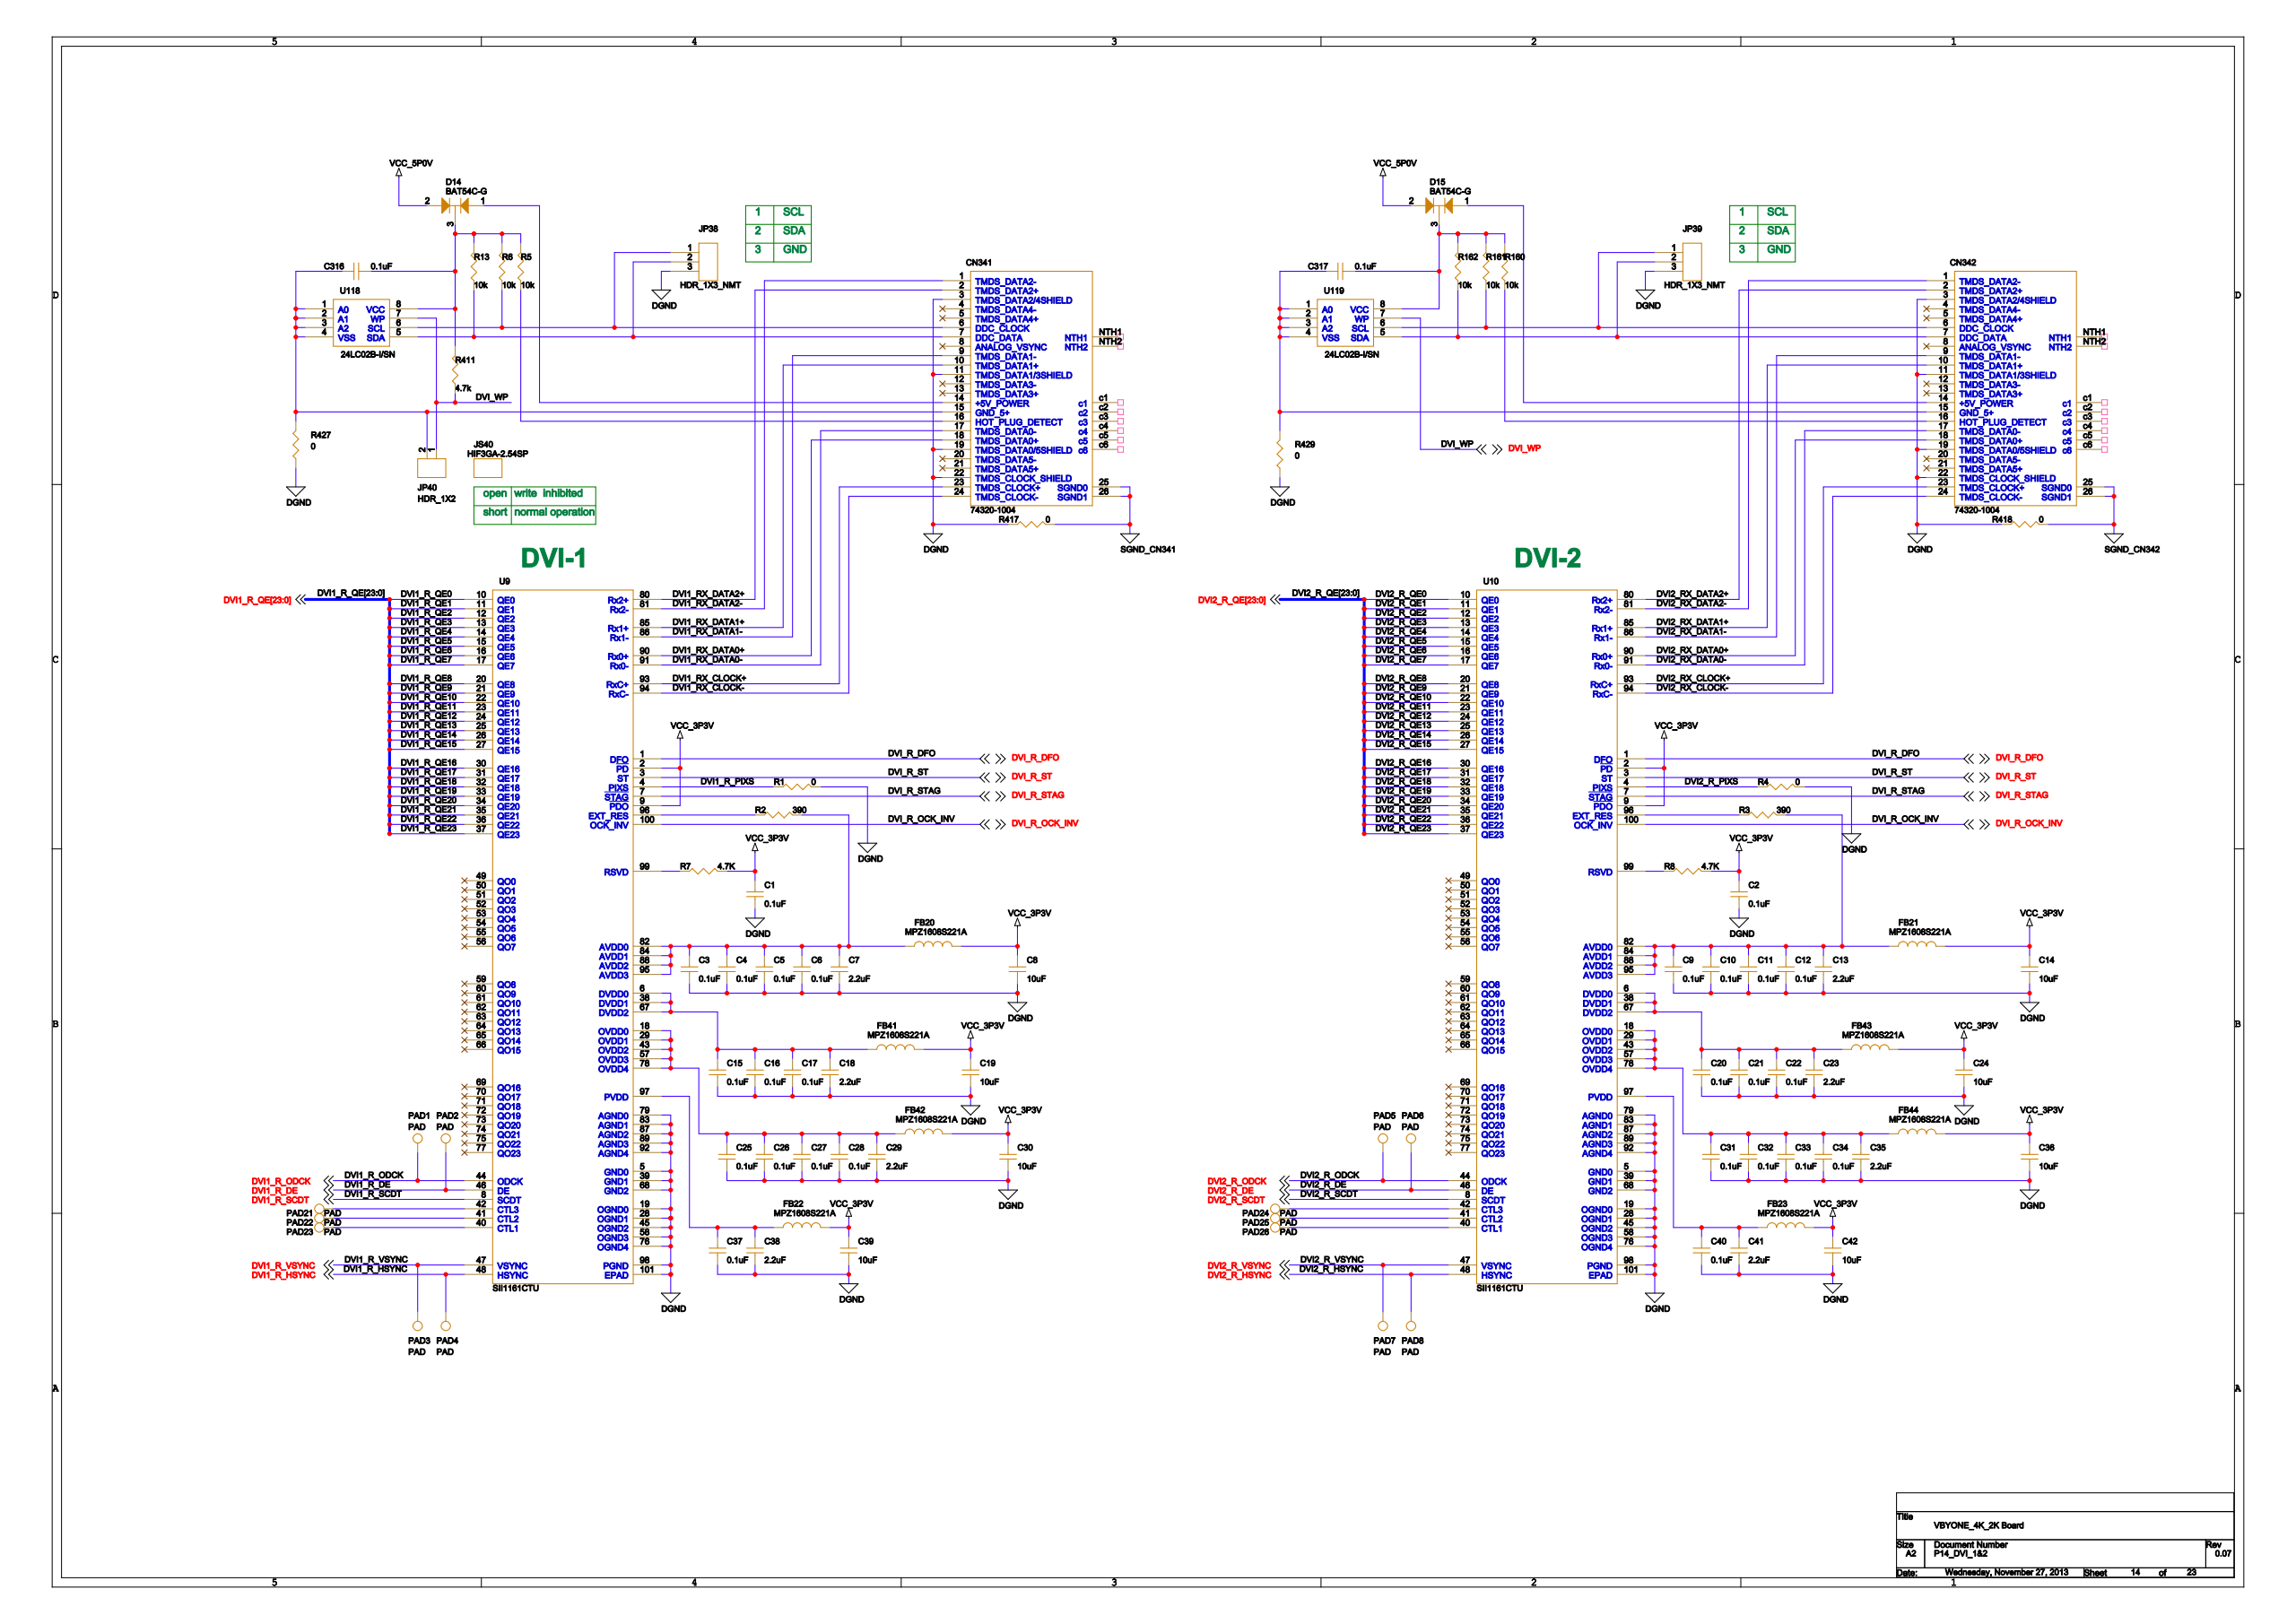Circuit board | Cadence Allegro | 1712 parts | 1495 nets | one sheet of the schematic
Parts on this sheet (reference | value | footprint):
C1 | 0.1uF | CRC1005RZAS
C2 | 0.1uF | CRC1005RZAS
C4 | 0.1uF | CRC1005RZAS
C5 | 0.1uF | CRC1005RZAS
C6 | 0.1uF | CRC1005RZAS
C8 | 10uF | CRC2012RZAS
C13 | 2.2uF | CRC1608RZAS
C14 | 10uF | CRC2012RZAS
C18 | 2.2uF | CRC1608RZAS
C19 | 10uF | CRC2012RZAS
C23 | 2.2uF | CRC1608RZAS
C24 | 10uF | CRC2012RZAS
C28 | 0.1uF | CRC1005RZAS
C29 | 2.2uF | CRC1608RZAS
C30 | 10uF | CRC2012RZAS
C31 | 0.1uF | CRC1005RZAS
C32 | 0.1uF | CRC1005RZAS
C33 | 0.1uF | CRC1005RZAS
C34 | 0.1uF | CRC1005RZAS
C35 | 2.2uF | CRC1608RZAS
C36 | 10uF | CRC2012RZAS
C37 | 0.1uF | CRC1005RZAS
C38 | 2.2uF | CRC1608RZAS
C39 | 10uF | CRC2012RZAS
C40 | 0.1uF | CRC1005RZAS
C41 | 2.2uF | CRC1608RZAS
C42 | 10uF | CRC2012RZAS
C316 | 0.1uF | CRC1005RZAS
C317 | 0.1uF | CRC1005RZAS
CN341 | 74320-1004 | CAD030LZAS
CN342 | 74320-1004 | CAD030LZAS
D14 | BAT54C-G | DIC003RZCS
D15 | BAT54C-G | DIC003RZCS
FB20 | MPZ1608S221A | LSC1608RZAS
FB21 | MPZ1608S221A | LSC1608RZAS
FB22 | MPZ1608S221A | LSC1608RZAS
FB23 | MPZ1608S221A | LSC1608RZAS
FB41 | MPZ1608S221A | LSC1608RZAS
FB42 | MPZ1608S221A | LSC1608RZAS
FB43 | MPZ1608S221A | LSC1608RZAS
FB44 | MPZ1608S221A | LSC1608RZAS
JP38 | HDR_1X3_NMT | CND003LLBS
JP39 | HDR_1X3_NMT | CND003LLBS
JP40 | HDR_1X2 | CND002LLBS
PAD1 | PAD | TPC050
PAD2 | PAD | TPC050
PAD3 | PAD | TPC050
PAD4 | PAD | TPC050
PAD5 | PAD | TPC050
PAD6 | PAD | TPC050
PAD7 | PAD | TPC050
PAD8 | PAD | TPC050
PAD21 | PAD | TPC050
PAD22 | PAD | TPC050
PAD23 | PAD | TPC050
PAD24 | PAD | TPC050
PAD25 | PAD | TPC050
PAD26 | PAD | TPC050
R1 | 0 | CRC1608RZAS
R2 | 390 | CRC1608RZAS
R3 | 390 | CRC1608RZAS
R4 | 0 | CRC1608RZAS
R160 | 10K | CRC1005RZAS
R161 | 10K | CRC1005RZAS
R162 | 10K | CRC1005RZAS
R411 | 4.7K | CRC1005RZAS
R417 | 0 | CRC1608RZAS
R418 | 0 | CRC1608RZAS
R427 | 0 | CRC1608RZAS
R429 | 0 | CRC1608RZAS
U9 | SII1161CTU | QFP100RCBS
U10 | SII1161CTU | QFP100RCBS
U118 | 24LC02B-I/SN | SOC008RHDS
U119 | 24LC02B-I/SN | SOC008RHDS
Nets of these parts (net: part-pin ...):
VCC_3P3V: C1-1 C2-1 C8-1 C14-1 C19-1 C24-1 C30-1 C36-1 C39-1 C42-1 FB20-2 FB21-2 FB22-2 FB23-2 FB41-2 FB42-2 FB43-2 FB44-2 U9-2 U9-9 U10-2 U10-9
DGND: C1-2 C2-2 C4-2 C5-2 C6-2 C8-2 C13-2 C14-2 C18-2 C19-2 C23-2 C24-2 C28-2 C29-2 C30-2 C31-2 C32-2 C33-2 C34-2 C35-2 C36-2 C37-2 C38-2 C39-2 C40-2 C41-2 C42-2 CN341-3 CN341-11 CN341-19 CN341-22 CN342-3 CN342-11 CN342-19 CN342-22 JP38-3 JP39-3 R1-2 R4-2 R417-1 R418-1 R427-1 R429-1 U9-5 U9-19 U9-28 U9-39 U9-45 U9-58 U9-68 U9-76 U9-79 U9-83 U9-87 U9-89 U9-92 U9-98 U9-101 U10-5 U10-19 U10-28 U10-39 U10-45 U10-58 U10-68 U10-76 U10-79 U10-83 U10-87 U10-89 U10-92 U10-98 U10-101
N15767478: C13-1 FB21-1 R3-2 U10-82 U10-84 U10-88 U10-95
N24349: C18-1 FB41-1 U9-6 U9-38 U9-67
N15766354: C23-1 FB43-1 U10-6 U10-38 U10-67
N24515: C28-1 C29-1 FB42-1 U9-18 U9-29 U9-43 U9-57 U9-78
N21036: C4-1 C5-1 C6-1 FB20-1 R2-2 U9-82 U9-84 U9-88 U9-95
N15766322: C31-1 C32-1 C33-1 C34-1 C35-1 FB44-1 U10-18 U10-29 U10-43 U10-57 U10-78
N18884444: C316-1 CN341-15 JP40-2 R427-2 U118-1 U118-2 U118-3 U118-4
N18884183: C316-2 D14-3 R411-2 U118-8
N18920873: C317-1 CN342-15 R429-2 U119-1 U119-2 U119-3 U119-4
N18920881: C317-2 D15-3 R160-2 R161-2 R162-2 U119-8
N24604: C37-1 C38-1 FB22-1 U9-97
N15768332: C40-1 C41-1 FB23-1 U10-97
VCC_5P0V: D14-2 D15-2
SGND_CN341: CN341-25 CN341-26 R417-2
DVI1_RX_DATA0-: CN341-17 U9-91
DVI1_RX_DATA1-: CN341-9 U9-86
DVI1_RX_DATA2-: CN341-1 U9-81
DVI1_RX_DATA0+: CN341-18 U9-90
DVI1_RX_DATA1+: CN341-10 U9-85
DVI1_RX_DATA2+: CN341-2 U9-80
N18886460: CN341-14 D14-1
N18884151: CN341-6 JP38-1 U118-6
DVI1_RX_CLOCK+: CN341-23 U9-93
N18884154: CN341-7 JP38-2 U118-5
DVI1_RX_CLOCK-: CN341-24 U9-94
N18884226: CN341-16
SGND_CN342: CN342-25 CN342-26 R418-2
DVI2_RX_DATA0-: CN342-17 U10-91
DVI2_RX_DATA1-: CN342-9 U10-86
DVI2_RX_DATA2-: CN342-1 U10-81
DVI2_RX_DATA0+: CN342-18 U10-90
DVI2_RX_DATA1+: CN342-10 U10-85
DVI2_RX_DATA2+: CN342-2 U10-80
N18920877: CN342-14 D15-1
N18920894: CN342-6 JP39-1 R161-1 U119-6
DVI2_RX_CLOCK+: CN342-23 U10-93
N18920900: CN342-7 JP39-2 R162-1 U119-5
DVI2_RX_CLOCK-: CN342-24 U10-94
N18921093: CN342-16 R160-1
DVI_WP: JP40-1 R411-1 U118-7 U119-7
DVI1_R_ODCK: PAD1-1 U9-44
DVI1_R_DE: PAD2-1 U9-46
N19424292: PAD21-1 U9-42
N19424320: PAD22-1 U9-41
N19424331: PAD23-1 U9-40
N19424363: PAD24-1 U10-42
N19424381: PAD25-1 U10-41
N19424379: PAD26-1 U10-40
DVI1_R_VSYNC: PAD3-1 U9-47
DVI1_R_HSYNC: PAD4-1 U9-48
DVI2_R_ODCK: PAD5-1 U10-44
DVI2_R_DE: PAD6-1 U10-46
DVI2_R_VSYNC: PAD7-1 U10-47
DVI2_R_HSYNC: PAD8-1 U10-48
DVI1_R_PIXS: R1-1 U9-4
DVI_R_OCK_INV: U9-100 U10-100
DVI2_R_PIXS: R4-1 U10-4
DVI_R_ST: U9-3 U10-3
DVI_R_DFO: U9-1 U10-1
N19368639: R2-1 U9-96
N19368223: R3-1 U10-96
DVI_R_STAG: U9-7 U10-7
DVI2_R_SCDT: U10-8
DVI2_R_QE0: U10-10
DVI2_R_QE2: U10-12
DVI2_R_QE1: U10-11
DVI2_R_QE3: U10-13
DVI2_R_QE4: U10-14
DVI2_R_QE6: U10-16
DVI2_R_QE5: U10-15
DVI2_R_QE7: U10-17
DVI2_R_QE8: U10-20
DVI2_R_QE9: U10-21
DVI2_R_QE10: U10-22
DVI2_R_QE12: U10-24
DVI2_R_QE11: U10-23
DVI2_R_QE13: U10-25
DVI2_R_QE14: U10-26
DVI2_R_QE15: U10-27
DVI2_R_QE16: U10-30
DVI2_R_QE17: U10-31
DVI2_R_QE19: U10-33
DVI2_R_QE18: U10-32
DVI2_R_QE20: U10-34
DVI2_R_QE21: U10-35
DVI2_R_QE23: U10-37
DVI2_R_QE22: U10-36
DVI1_R_SCDT: U9-8
DVI1_R_QE0: U9-10
DVI1_R_QE2: U9-12
DVI1_R_QE1: U9-11
DVI1_R_QE3: U9-13
DVI1_R_QE4: U9-14
DVI1_R_QE6: U9-16
DVI1_R_QE5: U9-15
DVI1_R_QE7: U9-17
DVI1_R_QE8: U9-20
DVI1_R_QE9: U9-21
DVI1_R_QE10: U9-22
DVI1_R_QE12: U9-24
DVI1_R_QE11: U9-23
DVI1_R_QE13: U9-25
DVI1_R_QE14: U9-26
DVI1_R_QE15: U9-27
DVI1_R_QE16: U9-30
DVI1_R_QE17: U9-31
DVI1_R_QE19: U9-33
DVI1_R_QE18: U9-32
DVI1_R_QE20: U9-34
DVI1_R_QE21: U9-35
DVI1_R_QE23: U9-37
DVI1_R_QE22: U9-36